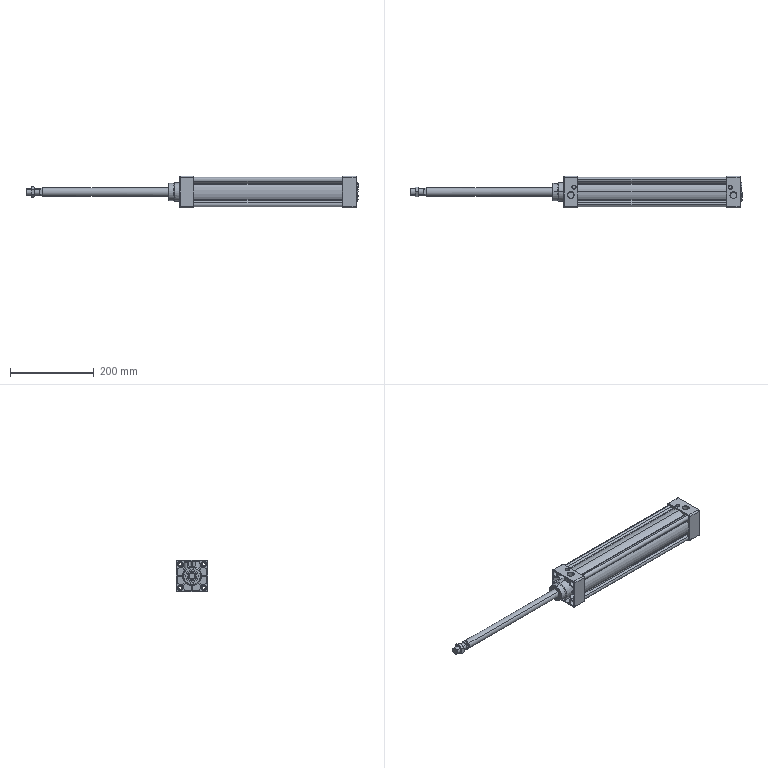Part | SolidWorks | 3 solids | 592 faces | box 792.217 x 75 x 75 mm | volume 831680 mm3 | plane 222 | cylinder 184 | cone 134 | spline 52 | commonest cylinder face diameters 12 x22 2.2 x18 8.7 x16 12.7 x16 7 x12 4 x10